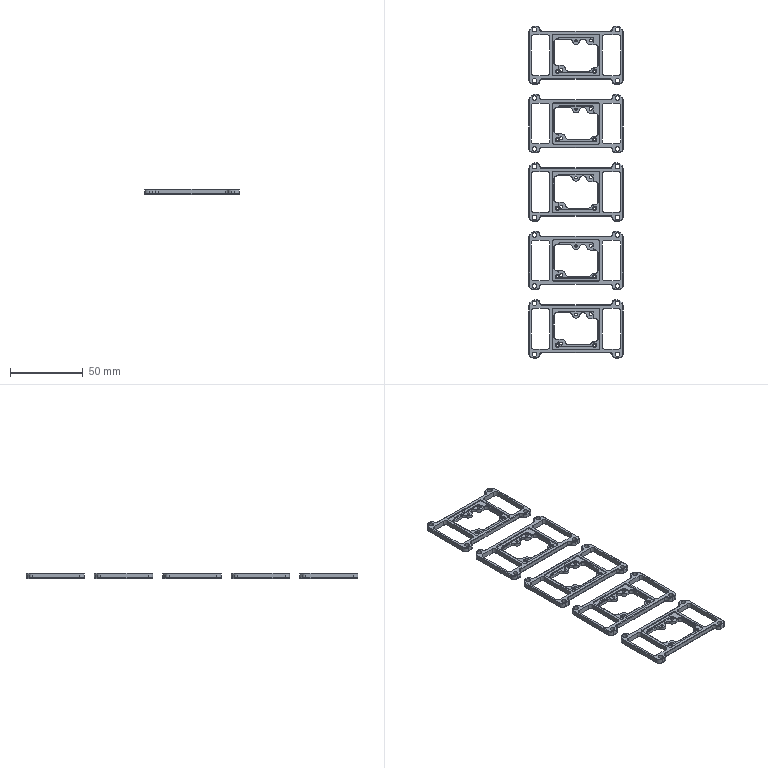NC program | NX | posted with a generic post | part box 65 x 228 x 3.5 mm
Lines 19 to 938 of 31259:
(ZLEVEL_PROFILE , TOOL : D6)
N36 T12 M6
N38 G54
N40 G17 G0 G90 X-57.9 Y21.227 S9500 M3
N42 G43 Z30. H12
N44 Z1.5
N46 G94 G1 Y20.975 Z1.487 F1000.
N48 X-36.1 Z0.344
N50 Y27.775 Z-0.012
N52 X-47. Z-0.583
N54 X-57.9 F3000.
N56 Y20.975
N58 X-36.1
N60 Y27.775
N62 X-47.
N64 X-57.9 Z-0.694
N66 Y20.975 Z-0.764
N68 X-36.1 Z-0.986
N70 Y27.775 Z-1.056
N72 X-47. Z-1.167
N74 X-57.9 Z-1.278
N76 Y20.975 Z-1.347
N78 X-36.1 Z-1.569
N80 Y27.775 Z-1.639
N82 X-47. Z-1.75
N84 X-57.9 Z-1.861
N86 Y20.975 Z-1.931
N88 X-36.1 Z-2.153
N90 Y27.775 Z-2.222
N92 X-47. Z-2.333
N94 X-57.9 Z-2.444
N96 Y20.975 Z-2.514
N98 X-36.1 Z-2.736
N100 Y27.775 Z-2.806
N102 X-47. Z-2.917
N104 X-57.9 Z-3.028
N106 Y20.975 Z-3.097
N108 X-36.1 Z-3.319
N110 Y27.775 Z-3.389
N112 X-47. Z-3.5
N114 X-57.9
N116 Y20.975
N118 X-36.1
N120 Y27.775
N122 X-47.
N124 Z-2.
N126 G0 Z53.
N128 X-36.1 Y-21.227
N130 Z1.5
N132 G1 Y-20.975 Z1.487 F1000.
N134 X-57.9 Z0.344
N136 Y-27.775 Z-0.012
N138 X-47. Z-0.583
N140 X-36.1 F3000.
N142 Y-20.975
N144 X-57.9
N146 Y-27.775
N148 X-47.
N150 X-36.1 Z-0.694
N152 Y-20.975 Z-0.764
N154 X-57.9 Z-0.986
N156 Y-27.775 Z-1.056
N158 X-47. Z-1.167
N160 X-36.1 Z-1.278
N162 Y-20.975 Z-1.347
N164 X-57.9 Z-1.569
N166 Y-27.775 Z-1.639
N168 X-47. Z-1.75
N170 X-36.1 Z-1.861
N172 Y-20.975 Z-1.931
N174 X-57.9 Z-2.153
N176 Y-27.775 Z-2.222
N178 X-47. Z-2.333
N180 X-36.1 Z-2.444
N182 Y-20.975 Z-2.514
N184 X-57.9 Z-2.736
N186 Y-27.775 Z-2.806
N188 X-47. Z-2.917
N190 X-36.1 Z-3.028
N192 Y-20.975 Z-3.097
N194 X-57.9 Z-3.319
N196 Y-27.775 Z-3.389
N198 X-47. Z-3.5
N200 X-36.1
N202 Y-20.975
N204 X-57.9
N206 Y-27.775
N208 X-47.
N210 Z-2.
N212 G0 Z53.
N214 X-44.696 Y11.9
N216 Z1.5
N218 G1 X-51. Z1.17 F1000.
N220 Y9.494 Z1.044
N222 X-51.262 Y8.23 Z0.976
N224 X-51.783 Y7.049 Z0.908
N226 X-52.54 Y6.003 Z0.841
N228 X-53.499 Y5.139 Z0.773
N230 X-54.022 Y4.834 Z0.741
N232 X-53.521 Y4.54 Z0.711
N234 X-52.481 Y3.551 Z0.636
N236 X-51.725 Y2.331 Z0.56
N238 X-51.302 Y0.959 Z0.485
N240 X-51.24 Y-0.475 Z0.41
N242 X-51.543 Y-1.878 Z0.335
N244 X-52.19 Y-3.159 Z0.259
N246 X-53.14 Y-4.235 Z0.184
N248 X-54.088 Y-4.906 Z0.123
N250 X-54.356 Y-5.047 Z0.107
N252 X-54.9 Y-5.25 Z0.077
N254 Y-11.9 Z-0.272
N256 X-48.95 Z-0.583
N258 X-43. F3000.
N260 Y-10.1
N262 G2 X-39.1 Y-4.411 R6.1
N264 G1 Y8.14
N266 G2 X-41.393 Y11.9 R5.6
N268 G1 X-51.
N270 Y10.1
N272 G2 X-54.022 Y4.834 R6.1
N274 X-54.9 Y-5.25 R5.6
N276 G1 Y-11.9
N278 X-48.95
N280 X-43. Z-0.63
N282 Y-10.1 Z-0.644
N284 X-42.978 Y-9.577 Z-0.648
N286 X-42.91 Y-9.058 Z-0.652
N288 X-42.799 Y-8.546 Z-0.656
N290 X-42.644 Y-8.046 Z-0.66
N292 X-42.447 Y-7.561 Z-0.664
N294 X-42.209 Y-7.095 Z-0.668
N296 X-41.931 Y-6.651 Z-0.672
N298 X-41.617 Y-6.232 Z-0.676
N300 X-41.268 Y-5.842 Z-0.68
N302 X-40.887 Y-5.483 Z-0.684
N304 X-40.477 Y-5.159 Z-0.688
N306 X-40.04 Y-4.87 Z-0.692
N308 X-39.586 Y-4.623 Z-0.696
N310 X-39.1 Y-4.411 Z-0.7
N312 Y8.14 Z-0.798
N314 X-39.549 Y8.495 Z-0.802
N316 X-39.949 Y8.885 Z-0.807
N318 X-40.313 Y9.318 Z-0.811
N320 X-40.631 Y9.785 Z-0.815
N322 X-40.901 Y10.282 Z-0.82
N324 X-41.119 Y10.804 Z-0.824
N326 X-41.281 Y11.335 Z-0.829
N328 X-41.393 Y11.9 Z-0.833
N330 X-51. Z-0.908
N332 Y10.1 Z-0.922
N334 X-51.023 Y9.571 Z-0.926
N336 X-51.092 Y9.046 Z-0.93
N338 X-51.206 Y8.529 Z-0.934
N340 X-51.364 Y8.024 Z-0.938
N342 X-51.566 Y7.534 Z-0.942
N344 X-51.809 Y7.064 Z-0.946
N346 X-52.092 Y6.617 Z-0.95
N348 X-52.413 Y6.196 Z-0.954
N350 X-52.77 Y5.804 Z-0.959
N352 X-53.158 Y5.445 Z-0.963
N354 X-53.566 Y5.128 Z-0.967
N356 X-54.022 Y4.834 Z-0.971
N358 X-53.542 Y4.518 Z-0.975
N360 X-53.12 Y4.177 Z-0.979
N362 X-52.722 Y3.784 Z-0.984
N364 X-52.366 Y3.354 Z-0.988
N366 X-52.054 Y2.891 Z-0.992
N368 X-51.79 Y2.398 Z-0.997
N370 X-51.576 Y1.882 Z-1.001
N372 X-51.414 Y1.347 Z-1.005
N374 X-51.307 Y0.799 Z-1.01
N376 X-51.255 Y0.243 Z-1.014
N378 X-51.259 Y-0.316 Z-1.018
N380 X-51.318 Y-0.871 Z-1.023
N382 X-51.433 Y-1.418 Z-1.027
N384 X-51.601 Y-1.951 Z-1.031
N386 X-51.821 Y-2.464 Z-1.036
N388 X-52.092 Y-2.953 Z-1.04
N390 X-52.41 Y-3.413 Z-1.044
N392 X-52.772 Y-3.838 Z-1.049
N394 X-53.175 Y-4.225 Z-1.053
N396 X-53.614 Y-4.57 Z-1.057
N398 X-53.918 Y-4.771 Z-1.06
N400 X-54.235 Y-4.952 Z-1.063
N402 X-54.559 Y-5.11 Z-1.066
N404 X-54.9 Y-5.25 Z-1.069
N406 Y-11.9 Z-1.12
N408 X-48.95 Z-1.167
N410 X-43. Z-1.213
N412 Y-10.1 Z-1.227
N414 X-42.978 Y-9.577 Z-1.231
N416 X-42.91 Y-9.058 Z-1.235
N418 X-42.799 Y-8.546 Z-1.239
N420 X-42.644 Y-8.046 Z-1.243
N422 X-42.447 Y-7.561 Z-1.247
N424 X-42.209 Y-7.095 Z-1.251
N426 X-41.931 Y-6.651 Z-1.255
N428 X-41.617 Y-6.232 Z-1.259
N430 X-41.268 Y-5.842 Z-1.263
N432 X-40.887 Y-5.483 Z-1.267
N434 X-40.477 Y-5.159 Z-1.272
N436 X-40.04 Y-4.87 Z-1.276
N438 X-39.586 Y-4.623 Z-1.28
N440 X-39.1 Y-4.411 Z-1.284
N442 Y8.14 Z-1.381
N444 X-39.549 Y8.495 Z-1.386
N446 X-39.949 Y8.885 Z-1.39
N448 X-40.313 Y9.318 Z-1.394
N450 X-40.631 Y9.785 Z-1.399
N452 X-40.901 Y10.282 Z-1.403
N454 X-41.119 Y10.804 Z-1.408
N456 X-41.281 Y11.335 Z-1.412
N458 X-41.393 Y11.9 Z-1.416
N460 X-51. Z-1.491
N462 Y10.1 Z-1.505
N464 X-51.023 Y9.571 Z-1.509
N466 X-51.092 Y9.046 Z-1.513
N468 X-51.206 Y8.529 Z-1.517
N470 X-51.364 Y8.024 Z-1.521
N472 X-51.566 Y7.534 Z-1.525
N474 X-51.809 Y7.064 Z-1.53
N476 X-52.092 Y6.617 Z-1.534
N478 X-52.413 Y6.196 Z-1.538
N480 X-52.77 Y5.804 Z-1.542
N482 X-53.158 Y5.445 Z-1.546
N484 X-53.566 Y5.128 Z-1.55
N486 X-54.022 Y4.834 Z-1.554
N488 X-53.542 Y4.518 Z-1.558
N490 X-53.12 Y4.177 Z-1.563
N492 X-52.722 Y3.784 Z-1.567
N494 X-52.366 Y3.354 Z-1.571
N496 X-52.054 Y2.891 Z-1.576
N498 X-51.79 Y2.398 Z-1.58
N500 X-51.576 Y1.882 Z-1.584
N502 X-51.414 Y1.347 Z-1.589
N504 X-51.307 Y0.799 Z-1.593
N506 X-51.255 Y0.243 Z-1.597
N508 X-51.259 Y-0.316 Z-1.602
N510 X-51.318 Y-0.871 Z-1.606
N512 X-51.433 Y-1.418 Z-1.61
N514 X-51.601 Y-1.951 Z-1.615
N516 X-51.821 Y-2.464 Z-1.619
N518 X-52.092 Y-2.953 Z-1.623
N520 X-52.41 Y-3.413 Z-1.628
N522 X-52.772 Y-3.838 Z-1.632
N524 X-53.175 Y-4.225 Z-1.636
N526 X-53.614 Y-4.57 Z-1.641
N528 X-53.918 Y-4.771 Z-1.644
N530 X-54.235 Y-4.952 Z-1.646
N532 X-54.559 Y-5.11 Z-1.649
N534 X-54.9 Y-5.25 Z-1.652
N536 Y-11.9 Z-1.704
N538 X-48.95 Z-1.75
N540 X-43. Z-1.796
N542 Y-10.1 Z-1.81
N544 X-42.978 Y-9.577 Z-1.814
N546 X-42.91 Y-9.058 Z-1.818
N548 X-42.799 Y-8.546 Z-1.822
N550 X-42.644 Y-8.046 Z-1.826
N552 X-42.447 Y-7.561 Z-1.83
N554 X-42.209 Y-7.095 Z-1.835
N556 X-41.931 Y-6.651 Z-1.839
N558 X-41.617 Y-6.232 Z-1.843
N560 X-41.268 Y-5.842 Z-1.847
N562 X-40.887 Y-5.483 Z-1.851
N564 X-40.477 Y-5.159 Z-1.855
N566 X-40.04 Y-4.87 Z-1.859
N568 X-39.586 Y-4.623 Z-1.863
N570 X-39.1 Y-4.411 Z-1.867
N572 Y8.14 Z-1.965
N574 X-39.549 Y8.495 Z-1.969
N576 X-39.949 Y8.885 Z-1.973
N578 X-40.313 Y9.318 Z-1.978
N580 X-40.631 Y9.785 Z-1.982
N582 X-40.901 Y10.282 Z-1.986
N584 X-41.119 Y10.804 Z-1.991
N586 X-41.281 Y11.335 Z-1.995
N588 X-41.393 Y11.9 Z-2.
N590 X-51. Z-2.074
N592 Y10.1 Z-2.088
N594 X-51.023 Y9.571 Z-2.092
N596 X-51.092 Y9.046 Z-2.096
N598 X-51.206 Y8.529 Z-2.101
N600 X-51.364 Y8.024 Z-2.105
N602 X-51.566 Y7.534 Z-2.109
N604 X-51.809 Y7.064 Z-2.113
N606 X-52.092 Y6.617 Z-2.117
N608 X-52.413 Y6.196 Z-2.121
N610 X-52.77 Y5.804 Z-2.125
N612 X-53.158 Y5.445 Z-2.129
N614 X-53.566 Y5.128 Z-2.133
N616 X-54.022 Y4.834 Z-2.137
N618 X-53.542 Y4.518 Z-2.142
N620 X-53.12 Y4.177 Z-2.146
N622 X-52.722 Y3.784 Z-2.15
N624 X-52.366 Y3.354 Z-2.155
N626 X-52.054 Y2.891 Z-2.159
N628 X-51.79 Y2.398 Z-2.163
N630 X-51.576 Y1.882 Z-2.168
N632 X-51.414 Y1.347 Z-2.172
N634 X-51.307 Y0.799 Z-2.176
N636 X-51.255 Y0.243 Z-2.181
N638 X-51.259 Y-0.316 Z-2.185
N640 X-51.318 Y-0.871 Z-2.189
N642 X-51.433 Y-1.418 Z-2.194
N644 X-51.601 Y-1.951 Z-2.198
N646 X-51.821 Y-2.464 Z-2.202
N648 X-52.092 Y-2.953 Z-2.207
N650 X-52.41 Y-3.413 Z-2.211
N652 X-52.772 Y-3.838 Z-2.215
N654 X-53.175 Y-4.225 Z-2.22
N656 X-53.614 Y-4.57 Z-2.224
N658 X-53.918 Y-4.771 Z-2.227
N660 X-54.235 Y-4.952 Z-2.23
N662 X-54.559 Y-5.11 Z-2.233
N664 X-54.9 Y-5.25 Z-2.235
N666 Y-11.9 Z-2.287
N668 X-48.95 Z-2.333
N670 X-43. Z-2.38
N672 Y-10.1 Z-2.394
N674 X-42.978 Y-9.577 Z-2.398
N676 X-42.91 Y-9.058 Z-2.402
N678 X-42.799 Y-8.546 Z-2.406
N680 X-42.644 Y-8.046 Z-2.41
N682 X-42.447 Y-7.561 Z-2.414
N684 X-42.209 Y-7.095 Z-2.418
N686 X-41.931 Y-6.651 Z-2.422
N688 X-41.617 Y-6.232 Z-2.426
N690 X-41.268 Y-5.842 Z-2.43
N692 X-40.887 Y-5.483 Z-2.434
N694 X-40.477 Y-5.159 Z-2.438
N696 X-40.04 Y-4.87 Z-2.442
N698 X-39.586 Y-4.623 Z-2.446
N700 X-39.1 Y-4.411 Z-2.45
N702 Y8.14 Z-2.548
N704 X-39.549 Y8.495 Z-2.552
N706 X-39.949 Y8.885 Z-2.557
N708 X-40.313 Y9.318 Z-2.561
N710 X-40.631 Y9.785 Z-2.565
N712 X-40.901 Y10.282 Z-2.57
N714 X-41.119 Y10.804 Z-2.574
N716 X-41.281 Y11.335 Z-2.579
N718 X-41.393 Y11.9 Z-2.583
N720 X-51. Z-2.658
N722 Y10.1 Z-2.672
N724 X-51.023 Y9.571 Z-2.676
N726 X-51.092 Y9.046 Z-2.68
N728 X-51.206 Y8.529 Z-2.684
N730 X-51.364 Y8.024 Z-2.688
N732 X-51.566 Y7.534 Z-2.692
N734 X-51.809 Y7.064 Z-2.696
N736 X-52.092 Y6.617 Z-2.7
N738 X-52.413 Y6.196 Z-2.704
N740 X-52.77 Y5.804 Z-2.709
N742 X-53.158 Y5.445 Z-2.713
N744 X-53.566 Y5.128 Z-2.717
N746 X-54.022 Y4.834 Z-2.721
N748 X-53.542 Y4.518 Z-2.725
N750 X-53.12 Y4.177 Z-2.729
N752 X-52.722 Y3.784 Z-2.734
N754 X-52.366 Y3.354 Z-2.738
N756 X-52.054 Y2.891 Z-2.742
N758 X-51.79 Y2.398 Z-2.747
N760 X-51.576 Y1.882 Z-2.751
N762 X-51.414 Y1.347 Z-2.755
N764 X-51.307 Y0.799 Z-2.76
N766 X-51.255 Y0.243 Z-2.764
N768 X-51.259 Y-0.316 Z-2.768
N770 X-51.318 Y-0.871 Z-2.773
N772 X-51.433 Y-1.418 Z-2.777
N774 X-51.601 Y-1.951 Z-2.781
N776 X-51.821 Y-2.464 Z-2.786
N778 X-52.092 Y-2.953 Z-2.79
N780 X-52.41 Y-3.413 Z-2.794
N782 X-52.772 Y-3.838 Z-2.799
N784 X-53.175 Y-4.225 Z-2.803
N786 X-53.614 Y-4.57 Z-2.807
N788 X-53.918 Y-4.771 Z-2.81
N790 X-54.235 Y-4.952 Z-2.813
N792 X-54.559 Y-5.11 Z-2.816
N794 X-54.9 Y-5.25 Z-2.819
N796 Y-11.9 Z-2.87
N798 X-48.95 Z-2.917
N800 X-43. Z-2.963
N802 Y-10.1 Z-2.977
N804 X-42.978 Y-9.577 Z-2.981
N806 X-42.91 Y-9.058 Z-2.985
N808 X-42.799 Y-8.546 Z-2.989
N810 X-42.644 Y-8.046 Z-2.993
N812 X-42.447 Y-7.561 Z-2.997
N814 X-42.209 Y-7.095 Z-3.001
N816 X-41.931 Y-6.651 Z-3.005
N818 X-41.617 Y-6.232 Z-3.009
N820 X-41.268 Y-5.842 Z-3.013
N822 X-40.887 Y-5.483 Z-3.017
N824 X-40.477 Y-5.159 Z-3.022
N826 X-40.04 Y-4.87 Z-3.026
N828 X-39.586 Y-4.623 Z-3.03
N830 X-39.1 Y-4.411 Z-3.034
N832 Y8.14 Z-3.131
N834 X-39.549 Y8.495 Z-3.136
N836 X-39.949 Y8.885 Z-3.14
N838 X-40.313 Y9.318 Z-3.144
N840 X-40.631 Y9.785 Z-3.149
N842 X-40.901 Y10.282 Z-3.153
N844 X-41.119 Y10.804 Z-3.158
N846 X-41.281 Y11.335 Z-3.162
N848 X-41.393 Y11.9 Z-3.166
N850 X-51. Z-3.241
N852 Y10.1 Z-3.255
N854 X-51.023 Y9.571 Z-3.259
N856 X-51.092 Y9.046 Z-3.263
N858 X-51.206 Y8.529 Z-3.267
N860 X-51.364 Y8.024 Z-3.271
N862 X-51.566 Y7.534 Z-3.275
N864 X-51.809 Y7.064 Z-3.28
N866 X-52.092 Y6.617 Z-3.284
N868 X-52.413 Y6.196 Z-3.288
N870 X-52.77 Y5.804 Z-3.292
N872 X-53.158 Y5.445 Z-3.296
N874 X-53.566 Y5.128 Z-3.3
N876 X-54.022 Y4.834 Z-3.304
N878 X-53.542 Y4.518 Z-3.308
N880 X-53.12 Y4.177 Z-3.313
N882 X-52.722 Y3.784 Z-3.317
N884 X-52.366 Y3.354 Z-3.321
N886 X-52.054 Y2.891 Z-3.326
N888 X-51.79 Y2.398 Z-3.33
N890 X-51.576 Y1.882 Z-3.334
N892 X-51.414 Y1.347 Z-3.339
N894 X-51.307 Y0.799 Z-3.343
N896 X-51.255 Y0.243 Z-3.347
N898 X-51.259 Y-0.316 Z-3.352
N900 X-51.318 Y-0.871 Z-3.356
N902 X-51.433 Y-1.418 Z-3.36
N904 X-51.601 Y-1.951 Z-3.365
N906 X-51.821 Y-2.464 Z-3.369
N908 X-52.092 Y-2.953 Z-3.373
N910 X-52.41 Y-3.413 Z-3.378
N912 X-52.772 Y-3.838 Z-3.382
N914 X-53.175 Y-4.225 Z-3.386
N916 X-53.614 Y-4.57 Z-3.391
N918 X-53.918 Y-4.771 Z-3.394
N920 X-54.235 Y-4.952 Z-3.396
N922 X-54.559 Y-5.11 Z-3.399
N924 X-54.9 Y-5.25 Z-3.402
N926 Y-11.9 Z-3.454
N928 X-48.95 Z-3.5
N930 X-43.
N932 Y-10.1
N934 G2 X-39.1 Y-4.411 R6.1
N936 G1 Y8.14
N938 G2 X-41.393 Y11.9 R5.6
N940 G1 X-51.
N942 Y10.1
N944 G2 X-54.022 Y4.834 R6.1
N946 X-54.9 Y-5.25 R5.6
N948 G1 Y-11.9
N950 X-48.95
N952 Z-2.
N954 G0 Z53.
N956 X-91.687 Y11.9
N958 Z1.5
N960 G1 X-98. Z1.169 F1000.
N962 Y9.494 Z1.043
N964 X-98.262 Y8.23 Z0.975
N966 X-98.783 Y7.049 Z0.908
N968 X-99.54 Y6.003 Z0.84
N970 X-100.499 Y5.139 Z0.772
N972 X-101.022 Y4.834 Z0.741
N974 X-100.521 Y4.54 Z0.71
N976 X-99.386 Y3.431 Z0.627
N978 X-98.606 Y2.049 Z0.544
N980 X-98.243 Y0.504 Z0.461
N982 X-98.325 Y-1.081 Z0.378
N984 X-98.846 Y-2.58 Z0.294
N986 X-99.765 Y-3.874 Z0.211
N988 X-101.009 Y-4.86 Z0.128
N990 X-101.716 Y-5.181 Z0.087
N992 X-101.9 Y-5.25 Z0.077
N994 Y-11.9 Z-0.272
N996 X-95.95 Z-0.583
N998 X-90. F3000.
N1000 Y-10.1
N1002 G2 X-86.1 Y-4.411 R6.1
N1004 G1 Y8.14
N1006 G2 X-88.393 Y11.9 R5.6
N1008 G1 X-98.
N1010 Y10.1
N1012 G2 X-101.022 Y4.834 R6.1
N1014 X-101.9 Y-5.25 R5.6
N1016 G1 Y-11.9
N1018 X-95.95
N1020 X-90. Z-0.63
N1022 Y-10.1 Z-0.644
N1024 X-89.978 Y-9.577 Z-0.648
N1026 X-89.91 Y-9.058 Z-0.652
N1028 X-89.799 Y-8.546 Z-0.656
N1030 X-89.644 Y-8.046 Z-0.66
N1032 X-89.447 Y-7.561 Z-0.664
N1034 X-89.209 Y-7.095 Z-0.668
N1036 X-88.931 Y-6.651 Z-0.672
N1038 X-88.617 Y-6.232 Z-0.676
N1040 X-88.268 Y-5.842 Z-0.68
N1042 X-87.887 Y-5.483 Z-0.684
N1044 X-87.477 Y-5.159 Z-0.688
N1046 X-87.04 Y-4.87 Z-0.692
N1048 X-86.586 Y-4.623 Z-0.696
N1050 X-86.1 Y-4.411 Z-0.7
N1052 Y8.14 Z-0.798
N1054 X-86.549 Y8.495 Z-0.802
N1056 X-86.949 Y8.885 Z-0.807
N1058 X-87.313 Y9.318 Z-0.811
N1060 X-87.631 Y9.785 Z-0.815
N1062 X-87.901 Y10.282 Z-0.82
N1064 X-88.119 Y10.804 Z-0.824
N1066 X-88.281 Y11.335 Z-0.829
N1068 X-88.393 Y11.9 Z-0.833
N1070 X-98. Z-0.908
N1072 Y10.1 Z-0.922
N1074 X-98.023 Y9.571 Z-0.926
N1076 X-98.092 Y9.046 Z-0.93
N1078 X-98.206 Y8.529 Z-0.934
N1080 X-98.364 Y8.024 Z-0.938
N1082 X-98.566 Y7.534 Z-0.942
N1084 X-98.809 Y7.064 Z-0.946
N1086 X-99.092 Y6.617 Z-0.95
N1088 X-99.413 Y6.196 Z-0.954
N1090 X-99.77 Y5.804 Z-0.959
N1092 X-100.158 Y5.445 Z-0.963
N1094 X-100.566 Y5.128 Z-0.967
N1096 X-101.022 Y4.834 Z-0.971
N1098 X-100.544 Y4.52 Z-0.975
N1100 X-100.123 Y4.18 Z-0.979
N1102 X-99.727 Y3.79 Z-0.984
N1104 X-99.371 Y3.362 Z-0.988
N1106 X-99.06 Y2.901 Z-0.992
N1108 X-98.796 Y2.411 Z-0.997
N1110 X-98.581 Y1.898 Z-1.001
N1112 X-98.419 Y1.366 Z-1.005
N1114 X-98.31 Y0.82 Z-1.01
N1116 X-98.256 Y0.266 Z-1.014
N1118 X-98.258 Y-0.29 Z-1.018
N1120 X-98.314 Y-0.844 Z-1.023
N1122 X-98.425 Y-1.389 Z-1.027
N1124 X-98.589 Y-1.92 Z-1.031
N1126 X-98.806 Y-2.433 Z-1.036
N1128 X-99.072 Y-2.921 Z-1.04
N1130 X-99.386 Y-3.381 Z-1.044
N1132 X-99.743 Y-3.807 Z-1.049
N1134 X-100.141 Y-4.196 Z-1.053
N1136 X-100.576 Y-4.543 Z-1.057
N1138 X-101.043 Y-4.845 Z-1.061
N1140 X-101.537 Y-5.1 Z-1.066
N1142 X-101.716 Y-5.178 Z-1.067
N1144 X-101.9 Y-5.25 Z-1.069
N1146 Y-11.9 Z-1.12
N1148 X-98.925 Z-1.144
N1150 X-95.95 Z-1.167
N1152 X-90. Z-1.213
N1154 Y-10.1 Z-1.227
N1156 X-89.978 Y-9.577 Z-1.231
N1158 X-89.91 Y-9.058 Z-1.235
N1160 X-89.799 Y-8.546 Z-1.239
N1162 X-89.644 Y-8.046 Z-1.243
N1164 X-89.447 Y-7.561 Z-1.247
N1166 X-89.209 Y-7.095 Z-1.251
N1168 X-88.931 Y-6.651 Z-1.255
N1170 X-88.617 Y-6.232 Z-1.259
N1172 X-88.268 Y-5.842 Z-1.263
N1174 X-87.887 Y-5.483 Z-1.267
N1176 X-87.477 Y-5.159 Z-1.272
N1178 X-87.04 Y-4.87 Z-1.276
N1180 X-86.586 Y-4.623 Z-1.28
N1182 X-86.1 Y-4.411 Z-1.284
N1184 Y8.14 Z-1.381
N1186 X-86.549 Y8.495 Z-1.386
N1188 X-86.949 Y8.885 Z-1.39
N1190 X-87.313 Y9.318 Z-1.394
N1192 X-87.631 Y9.785 Z-1.399
N1194 X-87.901 Y10.282 Z-1.403
N1196 X-88.119 Y10.804 Z-1.408
N1198 X-88.281 Y11.335 Z-1.412
N1200 X-88.393 Y11.9 Z-1.416
N1202 X-98. Z-1.491
N1204 Y10.1 Z-1.505
N1206 X-98.023 Y9.571 Z-1.509
N1208 X-98.092 Y9.046 Z-1.513
N1210 X-98.206 Y8.529 Z-1.517
N1212 X-98.364 Y8.024 Z-1.521
N1214 X-98.566 Y7.534 Z-1.525
N1216 X-98.809 Y7.064 Z-1.53
N1218 X-99.092 Y6.617 Z-1.534
N1220 X-99.413 Y6.196 Z-1.538
N1222 X-99.77 Y5.804 Z-1.542
N1224 X-100.158 Y5.445 Z-1.546
N1226 X-100.566 Y5.128 Z-1.55
N1228 X-101.022 Y4.834 Z-1.554
N1230 X-100.544 Y4.52 Z-1.558
N1232 X-100.123 Y4.18 Z-1.563
N1234 X-99.727 Y3.79 Z-1.567
N1236 X-99.371 Y3.362 Z-1.571
N1238 X-99.06 Y2.901 Z-1.576
N1240 X-98.796 Y2.411 Z-1.58
N1242 X-98.581 Y1.898 Z-1.584
N1244 X-98.419 Y1.366 Z-1.589
N1246 X-98.31 Y0.82 Z-1.593
N1248 X-98.256 Y0.266 Z-1.597
N1250 X-98.258 Y-0.29 Z-1.602
N1252 X-98.314 Y-0.844 Z-1.606
N1254 X-98.425 Y-1.389 Z-1.61
N1256 X-98.589 Y-1.92 Z-1.615
N1258 X-98.806 Y-2.433 Z-1.619
N1260 X-99.072 Y-2.921 Z-1.623
N1262 X-99.386 Y-3.381 Z-1.628
N1264 X-99.743 Y-3.807 Z-1.632
N1266 X-100.141 Y-4.196 Z-1.636
N1268 X-100.576 Y-4.543 Z-1.64
N1270 X-101.043 Y-4.845 Z-1.645
N1272 X-101.537 Y-5.1 Z-1.649
N1274 X-101.716 Y-5.178 Z-1.651
N1276 X-101.9 Y-5.25 Z-1.652
N1278 Y-11.9 Z-1.704
N1280 X-98.925 Z-1.727
N1282 X-95.95 Z-1.75
N1284 X-90. Z-1.796
N1286 Y-10.1 Z-1.81
N1288 X-89.978 Y-9.577 Z-1.814
N1290 X-89.91 Y-9.058 Z-1.818
N1292 X-89.799 Y-8.546 Z-1.822
N1294 X-89.644 Y-8.046 Z-1.826
N1296 X-89.447 Y-7.561 Z-1.83
N1298 X-89.209 Y-7.095 Z-1.835
N1300 X-88.931 Y-6.651 Z-1.839
N1302 X-88.617 Y-6.232 Z-1.843
N1304 X-88.268 Y-5.842 Z-1.847
N1306 X-87.887 Y-5.483 Z-1.851
N1308 X-87.477 Y-5.159 Z-1.855
N1310 X-87.04 Y-4.87 Z-1.859
N1312 X-86.586 Y-4.623 Z-1.863
N1314 X-86.1 Y-4.411 Z-1.867
N1316 Y8.14 Z-1.965
N1318 X-86.549 Y8.495 Z-1.969
N1320 X-86.949 Y8.885 Z-1.973
N1322 X-87.313 Y9.318 Z-1.978
N1324 X-87.631 Y9.785 Z-1.982
N1326 X-87.901 Y10.282 Z-1.986
N1328 X-88.119 Y10.804 Z-1.991
N1330 X-88.281 Y11.335 Z-1.995
N1332 X-88.393 Y11.9 Z-2.
N1334 X-98. Z-2.074
N1336 Y10.1 Z-2.088
N1338 X-98.023 Y9.571 Z-2.092
N1340 X-98.092 Y9.046 Z-2.096
N1342 X-98.206 Y8.529 Z-2.101
N1344 X-98.364 Y8.024 Z-2.105
N1346 X-98.566 Y7.534 Z-2.109
N1348 X-98.809 Y7.064 Z-2.113
N1350 X-99.092 Y6.617 Z-2.117
N1352 X-99.413 Y6.196 Z-2.121
N1354 X-99.77 Y5.804 Z-2.125
N1356 X-100.158 Y5.445 Z-2.129
N1358 X-100.566 Y5.128 Z-2.133
N1360 X-101.022 Y4.834 Z-2.137
N1362 X-100.544 Y4.52 Z-2.142
N1364 X-100.123 Y4.18 Z-2.146
N1366 X-99.727 Y3.79 Z-2.15
N1368 X-99.371 Y3.362 Z-2.155
N1370 X-99.06 Y2.901 Z-2.159
N1372 X-98.796 Y2.411 Z-2.163
N1374 X-98.581 Y1.898 Z-2.168
N1376 X-98.419 Y1.366 Z-2.172
N1378 X-98.31 Y0.82 Z-2.176
N1380 X-98.256 Y0.266 Z-2.181
N1382 X-98.258 Y-0.29 Z-2.185
N1384 X-98.314 Y-0.844 Z-2.189
N1386 X-98.425 Y-1.389 Z-2.194
N1388 X-98.589 Y-1.92 Z-2.198
N1390 X-98.806 Y-2.433 Z-2.202
N1392 X-99.072 Y-2.921 Z-2.207
N1394 X-99.386 Y-3.381 Z-2.211
N1396 X-99.743 Y-3.807 Z-2.215
N1398 X-100.141 Y-4.196 Z-2.219
N1400 X-100.576 Y-4.543 Z-2.224
N1402 X-101.043 Y-4.845 Z-2.228
N1404 X-101.537 Y-5.1 Z-2.232
N1406 X-101.716 Y-5.178 Z-2.234
N1408 X-101.9 Y-5.25 Z-2.235
N1410 Y-11.9 Z-2.287
N1412 X-98.925 Z-2.31
N1414 X-95.95 Z-2.333
N1416 X-90. Z-2.38
N1418 Y-10.1 Z-2.394
N1420 X-89.978 Y-9.577 Z-2.398
N1422 X-89.91 Y-9.058 Z-2.402
N1424 X-89.799 Y-8.546 Z-2.406
N1426 X-89.644 Y-8.046 Z-2.41
N1428 X-89.447 Y-7.561 Z-2.414
N1430 X-89.209 Y-7.095 Z-2.418
N1432 X-88.931 Y-6.651 Z-2.422
N1434 X-88.617 Y-6.232 Z-2.426
N1436 X-88.268 Y-5.842 Z-2.43
N1438 X-87.887 Y-5.483 Z-2.434
N1440 X-87.477 Y-5.159 Z-2.438
N1442 X-87.04 Y-4.87 Z-2.442
N1444 X-86.586 Y-4.623 Z-2.446
N1446 X-86.1 Y-4.411 Z-2.45
N1448 Y8.14 Z-2.548
N1450 X-86.549 Y8.495 Z-2.552
N1452 X-86.949 Y8.885 Z-2.557
N1454 X-87.313 Y9.318 Z-2.561
N1456 X-87.631 Y9.785 Z-2.565
N1458 X-87.901 Y10.282 Z-2.57
N1460 X-88.119 Y10.804 Z-2.574
N1462 X-88.281 Y11.335 Z-2.579
N1464 X-88.393 Y11.9 Z-2.583
N1466 X-98. Z-2.658
N1468 Y10.1 Z-2.672
N1470 X-98.023 Y9.571 Z-2.676
N1472 X-98.092 Y9.046 Z-2.68
N1474 X-98.206 Y8.529 Z-2.684
N1476 X-98.364 Y8.024 Z-2.688
N1478 X-98.566 Y7.534 Z-2.692
N1480 X-98.809 Y7.064 Z-2.696
N1482 X-99.092 Y6.617 Z-2.7
N1484 X-99.413 Y6.196 Z-2.704
N1486 X-99.77 Y5.804 Z-2.709
N1488 X-100.158 Y5.445 Z-2.713
N1490 X-100.566 Y5.128 Z-2.717
N1492 X-101.022 Y4.834 Z-2.721
N1494 X-100.544 Y4.52 Z-2.725
N1496 X-100.123 Y4.18 Z-2.729
N1498 X-99.727 Y3.79 Z-2.734
N1500 X-99.371 Y3.362 Z-2.738
N1502 X-99.06 Y2.901 Z-2.742
N1504 X-98.796 Y2.411 Z-2.747
N1506 X-98.581 Y1.898 Z-2.751
N1508 X-98.419 Y1.366 Z-2.755
N1510 X-98.31 Y0.82 Z-2.76
N1512 X-98.256 Y0.266 Z-2.764
N1514 X-98.258 Y-0.29 Z-2.768
N1516 X-98.314 Y-0.844 Z-2.773
N1518 X-98.425 Y-1.389 Z-2.777
N1520 X-98.589 Y-1.92 Z-2.781
N1522 X-98.806 Y-2.433 Z-2.786
N1524 X-99.072 Y-2.921 Z-2.79
N1526 X-99.386 Y-3.381 Z-2.794
N1528 X-99.743 Y-3.807 Z-2.799
N1530 X-100.141 Y-4.196 Z-2.803
N1532 X-100.576 Y-4.543 Z-2.807
N1534 X-101.043 Y-4.845 Z-2.811
N1536 X-101.537 Y-5.1 Z-2.816
N1538 X-101.716 Y-5.178 Z-2.817
N1540 X-101.9 Y-5.25 Z-2.819
N1542 Y-11.9 Z-2.87
N1544 X-98.925 Z-2.894
N1546 X-95.95 Z-2.917
N1548 X-90. Z-2.963
N1550 Y-10.1 Z-2.977
N1552 X-89.978 Y-9.577 Z-2.981
N1554 X-89.91 Y-9.058 Z-2.985
N1556 X-89.799 Y-8.546 Z-2.989
N1558 X-89.644 Y-8.046 Z-2.993
N1560 X-89.447 Y-7.561 Z-2.997
N1562 X-89.209 Y-7.095 Z-3.001
N1564 X-88.931 Y-6.651 Z-3.005
N1566 X-88.617 Y-6.232 Z-3.009
N1568 X-88.268 Y-5.842 Z-3.013
N1570 X-87.887 Y-5.483 Z-3.017
N1572 X-87.477 Y-5.159 Z-3.022
N1574 X-87.04 Y-4.87 Z-3.026
N1576 X-86.586 Y-4.623 Z-3.03
N1578 X-86.1 Y-4.411 Z-3.034
N1580 Y8.14 Z-3.131
N1582 X-86.549 Y8.495 Z-3.136
N1584 X-86.949 Y8.885 Z-3.14
N1586 X-87.313 Y9.318 Z-3.144
N1588 X-87.631 Y9.785 Z-3.149
N1590 X-87.901 Y10.282 Z-3.153
N1592 X-88.119 Y10.804 Z-3.158
N1594 X-88.281 Y11.335 Z-3.162
N1596 X-88.393 Y11.9 Z-3.166
N1598 X-98. Z-3.241
N1600 Y10.1 Z-3.255
N1602 X-98.023 Y9.571 Z-3.259
N1604 X-98.092 Y9.046 Z-3.263
N1606 X-98.206 Y8.529 Z-3.267
N1608 X-98.364 Y8.024 Z-3.271
N1610 X-98.566 Y7.534 Z-3.275
N1612 X-98.809 Y7.064 Z-3.28
N1614 X-99.092 Y6.617 Z-3.284
N1616 X-99.413 Y6.196 Z-3.288
N1618 X-99.77 Y5.804 Z-3.292
N1620 X-100.158 Y5.445 Z-3.296
N1622 X-100.566 Y5.128 Z-3.3
N1624 X-101.022 Y4.834 Z-3.304
N1626 X-100.544 Y4.52 Z-3.308
N1628 X-100.123 Y4.18 Z-3.313
N1630 X-99.727 Y3.79 Z-3.317
N1632 X-99.371 Y3.362 Z-3.321
N1634 X-99.06 Y2.901 Z-3.326
N1636 X-98.796 Y2.411 Z-3.33
N1638 X-98.581 Y1.898 Z-3.334
N1640 X-98.419 Y1.366 Z-3.339
N1642 X-98.31 Y0.82 Z-3.343
N1644 X-98.256 Y0.266 Z-3.347
N1646 X-98.258 Y-0.29 Z-3.352
N1648 X-98.314 Y-0.844 Z-3.356
N1650 X-98.425 Y-1.389 Z-3.36
N1652 X-98.589 Y-1.92 Z-3.365
N1654 X-98.806 Y-2.433 Z-3.369
N1656 X-99.072 Y-2.921 Z-3.373
N1658 X-99.386 Y-3.381 Z-3.378
N1660 X-99.743 Y-3.807 Z-3.382
N1662 X-100.141 Y-4.196 Z-3.386
N1664 X-100.576 Y-4.543 Z-3.39
N1666 X-101.043 Y-4.845 Z-3.395
N1668 X-101.537 Y-5.1 Z-3.399
N1670 X-101.716 Y-5.178 Z-3.401
N1672 X-101.9 Y-5.25 Z-3.402
N1674 Y-11.9 Z-3.454
N1676 X-98.925 Z-3.477
N1678 X-95.95 Z-3.5
N1680 X-90.
N1682 Y-10.1
N1684 G2 X-86.1 Y-4.411 R6.1
N1686 G1 Y8.14
N1688 G2 X-88.393 Y11.9 R5.6
N1690 G1 X-98.
N1692 Y10.1
N1694 G2 X-101.022 Y4.834 R6.1
N1696 X-101.9 Y-5.25 R5.6
N1698 G1 Y-11.9
N1700 X-95.95
N1702 Z-2.
N1704 G0 Z53.
N1706 X-104.9 Y21.227
N1708 Z1.5
N1710 G1 Y20.975 Z1.487 F1000.
N1712 X-83.1 Z0.344
N1714 Y27.775 Z-0.012
N1716 X-94. Z-0.583
N1718 X-104.9 F3000.
N1720 Y20.975
N1722 X-83.1
N1724 Y27.775
N1726 X-94.
N1728 X-104.9 Z-0.694
N1730 Y20.975 Z-0.764
N1732 X-88.55 Z-0.931
N1734 X-85.825 Z-0.958
N1736 X-83.1 Z-0.986
N1738 Y27.775 Z-1.056
N1740 X-94. Z-1.167
N1742 X-104.9 Z-1.278
N1744 Y20.975 Z-1.347
N1746 X-88.55 Z-1.514
N1748 X-85.825 Z-1.542
N1750 X-83.1 Z-1.569
N1752 Y27.775 Z-1.639
N1754 X-94. Z-1.75
N1756 X-104.9 Z-1.861
N1758 Y20.975 Z-1.931
N1760 X-88.55 Z-2.097
N1762 X-85.825 Z-2.125
N1764 X-83.1 Z-2.153
N1766 Y27.775 Z-2.222
N1768 X-94. Z-2.333
N1770 X-104.9 Z-2.444
N1772 Y20.975 Z-2.514
N1774 X-88.55 Z-2.681
N1776 X-85.825 Z-2.708
N1778 X-83.1 Z-2.736
N1780 Y27.775 Z-2.806
N1782 X-94. Z-2.917
N1784 X-104.9 Z-3.028
N1786 Y20.975 Z-3.097
N1788 X-88.55 Z-3.264
N1790 X-85.825 Z-3.292
N1792 X-83.1 Z-3.319
N1794 Y27.775 Z-3.389
N1796 X-94. Z-3.5
N1798 X-104.9
N1800 Y20.975
N1802 X-83.1
N1804 Y27.775
N1806 X-94.
N1808 Z-2.
N1810 G0 Z53.
N1812 X-83.1 Y-21.227
N1814 Z1.5
N1816 G1 Y-20.975 Z1.487 F1000.
N1818 X-104.9 Z0.344
N1820 Y-27.775 Z-0.012
N1822 X-94. Z-0.583
N1824 X-83.1 F3000.
N1826 Y-20.975
N1828 X-104.9
N1830 Y-27.775
N1832 X-94.
N1834 X-83.1 Z-0.694
N1836 Y-20.975 Z-0.764
N1838 X-85.825 Z-0.792
N1840 X-88.55 Z-0.819
N1842 X-104.9 Z-0.986
N1844 Y-27.775 Z-1.056
N1846 X-94. Z-1.167
N1848 X-83.1 Z-1.278
N1850 Y-20.975 Z-1.347
N1852 X-85.825 Z-1.375
N1854 X-88.55 Z-1.403
N1856 X-104.9 Z-1.569
N1858 Y-27.775 Z-1.639
N1860 X-94. Z-1.75
N1862 X-83.1 Z-1.861
N1864 Y-20.975 Z-1.931
N1866 X-85.825 Z-1.958
N1868 X-88.55 Z-1.986